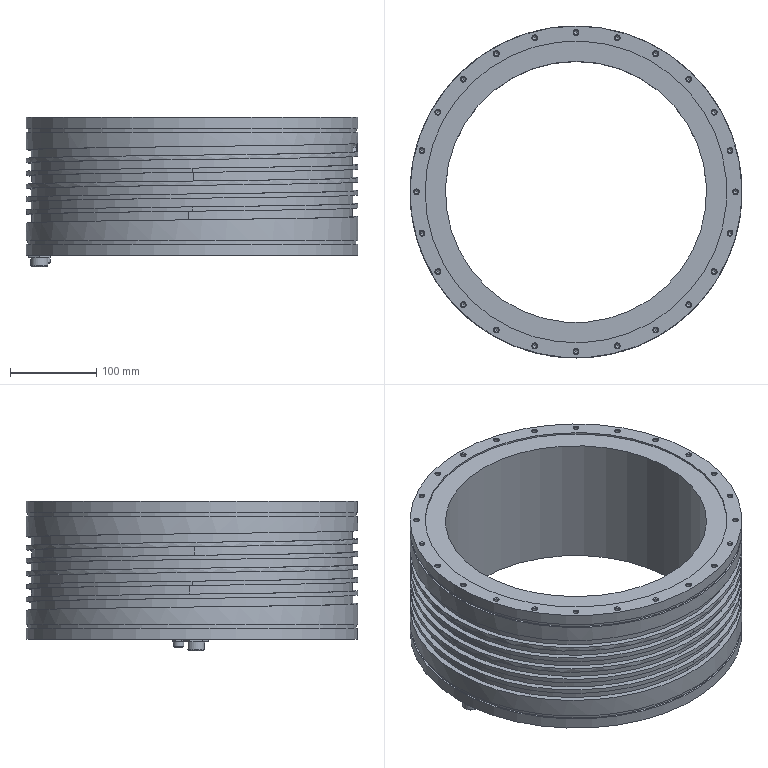Part | STEP file | Stator | 1 solid | 222 faces | box 385 x 385 x 173 mm | volume 6529567 mm3 | cone 98 | cylinder 80 | plane 38 | spline 6 | commonest cylinder face diameters 4.917 x48 385 x10 373 x8 350 x3 10 x2 381 x2